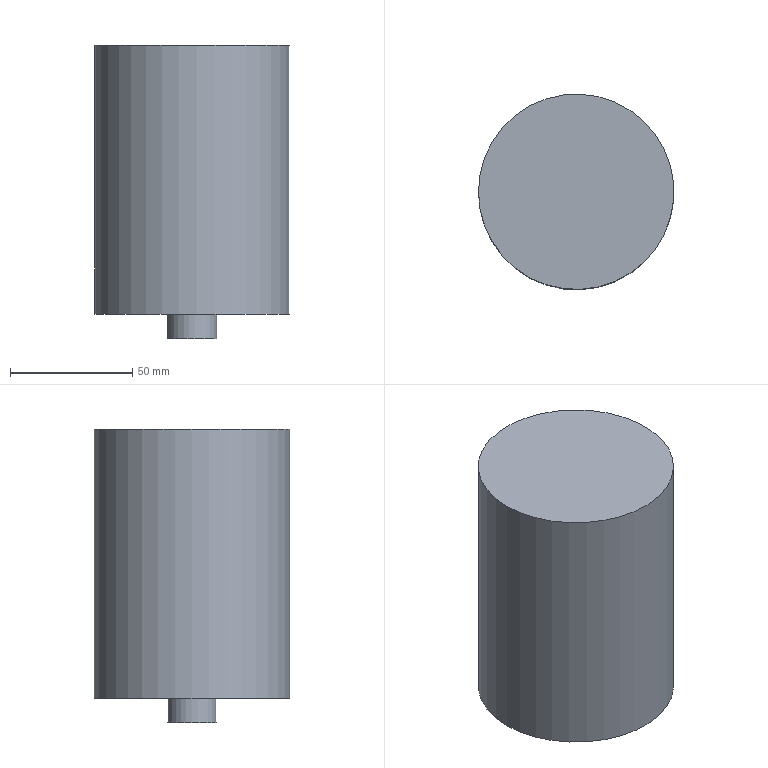Part | NX | features solid 2 | 1 solid | 5 faces | box 80 x 80 x 120 mm | volume 556062 mm3 | plane 3 | cylinder 2 | commonest cylinder face diameters 20 x1 80 x1
STEP:
#1=CARTESIAN_POINT('',(900.,-195.,-41.));
#2=VERTEX_POINT('',#1);
#3=CARTESIAN_POINT('',(940.,-195.,-41.));
#4=DIRECTION('',(0.,0.,-1.));
#5=DIRECTION('',(-1.,0.,0.));
#6=AXIS2_PLACEMENT_3D('',#3,#4,#5);
#7=CIRCLE('',#6,40.);
#8=EDGE_CURVE('',#2,#2,#7,.T.);
#9=ORIENTED_EDGE('',*,*,#8,.T.);
#10=EDGE_LOOP('',(#9));
#11=FACE_BOUND('',#10,.T.);
#12=CARTESIAN_POINT('',(900.,-195.,-151.));
#13=VERTEX_POINT('',#12);
#14=CARTESIAN_POINT('',(940.,-195.,-151.));
#15=DIRECTION('',(0.,0.,1.));
#16=DIRECTION('',(-1.,0.,0.));
#17=AXIS2_PLACEMENT_3D('',#14,#15,#16);
#18=CIRCLE('',#17,40.);
#19=EDGE_CURVE('',#13,#13,#18,.F.);
#20=ORIENTED_EDGE('',*,*,#19,.F.);
#21=EDGE_LOOP('',(#20));
#22=FACE_BOUND('',#21,.T.);
#23=CARTESIAN_POINT('',(940.,-195.,-91.));
#24=DIRECTION('',(0.,0.,-1.));
#25=DIRECTION('',(1.,0.,0.));
#26=AXIS2_PLACEMENT_3D('',#23,#24,#25);
#27=CYLINDRICAL_SURFACE('',#26,40.);
#28=ADVANCED_FACE('',(#11,#22),#27,.T.);
#29=ORIENTED_EDGE('',*,*,#8,.F.);
#30=EDGE_LOOP('',(#29));
#31=FACE_BOUND('',#30,.T.);
#32=CARTESIAN_POINT('',(-940.,715.,-41.));
#33=DIRECTION('',(0.,0.,-1.));
#34=DIRECTION('',(-1.,0.,0.));
#35=AXIS2_PLACEMENT_3D('',#32,#33,#34);
#36=PLANE('',#35);
#37=ADVANCED_FACE('',(#31),#36,.F.);
#38=CARTESIAN_POINT('',(950.,-195.,-151.));
#39=VERTEX_POINT('',#38);
#40=CARTESIAN_POINT('',(940.,-195.,-151.));
#41=DIRECTION('',(0.,0.,-1.));
#42=DIRECTION('',(1.,0.,0.));
#43=AXIS2_PLACEMENT_3D('',#40,#41,#42);
#44=CIRCLE('',#43,10.);
#45=EDGE_CURVE('',#39,#39,#44,.T.);
#46=ORIENTED_EDGE('',*,*,#45,.F.);
#47=EDGE_LOOP('',(#46));
#48=FACE_BOUND('',#47,.T.);
#49=ORIENTED_EDGE('',*,*,#19,.T.);
#50=EDGE_LOOP('',(#49));
#51=FACE_BOUND('',#50,.T.);
#52=CARTESIAN_POINT('',(940.,-195.,-151.));
#53=DIRECTION('',(0.,0.,-1.));
#54=DIRECTION('',(1.,0.,0.));
#55=AXIS2_PLACEMENT_3D('',#52,#53,#54);
#56=PLANE('',#55);
#57=ADVANCED_FACE('',(#48,#51),#56,.T.);
#58=ORIENTED_EDGE('',*,*,#45,.T.);
#59=EDGE_LOOP('',(#58));
#60=FACE_BOUND('',#59,.T.);
#61=CARTESIAN_POINT('',(950.,-195.,-161.));
#62=VERTEX_POINT('',#61);
#63=CARTESIAN_POINT('',(940.,-195.,-161.));
#64=DIRECTION('',(0.,0.,-1.));
#65=DIRECTION('',(1.,0.,0.));
#66=AXIS2_PLACEMENT_3D('',#63,#64,#65);
#67=CIRCLE('',#66,10.);
#68=EDGE_CURVE('',#62,#62,#67,.T.);
#69=ORIENTED_EDGE('',*,*,#68,.F.);
#70=EDGE_LOOP('',(#69));
#71=FACE_BOUND('',#70,.T.);
#72=CARTESIAN_POINT('',(940.,-195.,-151.));
#73=DIRECTION('',(0.,0.,-1.));
#74=DIRECTION('',(1.,0.,0.));
#75=AXIS2_PLACEMENT_3D('',#72,#73,#74);
#76=CYLINDRICAL_SURFACE('',#75,10.);
#77=ADVANCED_FACE('',(#60,#71),#76,.T.);
#78=ORIENTED_EDGE('',*,*,#68,.T.);
#79=EDGE_LOOP('',(#78));
#80=FACE_BOUND('',#79,.T.);
#81=CARTESIAN_POINT('',(940.,-195.,-161.));
#82=DIRECTION('',(0.,0.,-1.));
#83=DIRECTION('',(1.,0.,0.));
#84=AXIS2_PLACEMENT_3D('',#81,#82,#83);
#85=PLANE('',#84);
#86=ADVANCED_FACE('',(#80),#85,.T.);
#87=CLOSED_SHELL('',(#28,#37,#57,#77,#86));
#88=MANIFOLD_SOLID_BREP('',#87);
#89=(LENGTH_UNIT()NAMED_UNIT(*)SI_UNIT(.MILLI.,.METRE.));
#90=UNCERTAINTY_MEASURE_WITH_UNIT(LENGTH_MEASURE(0.00001),#89,'','');
#91=(NAMED_UNIT(*)PLANE_ANGLE_UNIT()SI_UNIT($,.RADIAN.));
#92=(NAMED_UNIT(*)SI_UNIT($,.STERADIAN.)SOLID_ANGLE_UNIT());
#93=(GEOMETRIC_REPRESENTATION_CONTEXT(3)GLOBAL_UNCERTAINTY_ASSIGNED_CONTEXT((#90))GLOBAL_UNIT_ASSIGNED_CONTEXT((#89,#91,#92))REPRESENTATION_CONTEXT('',''));
#94=ADVANCED_BREP_SHAPE_REPRESENTATION('',(#88),#93);